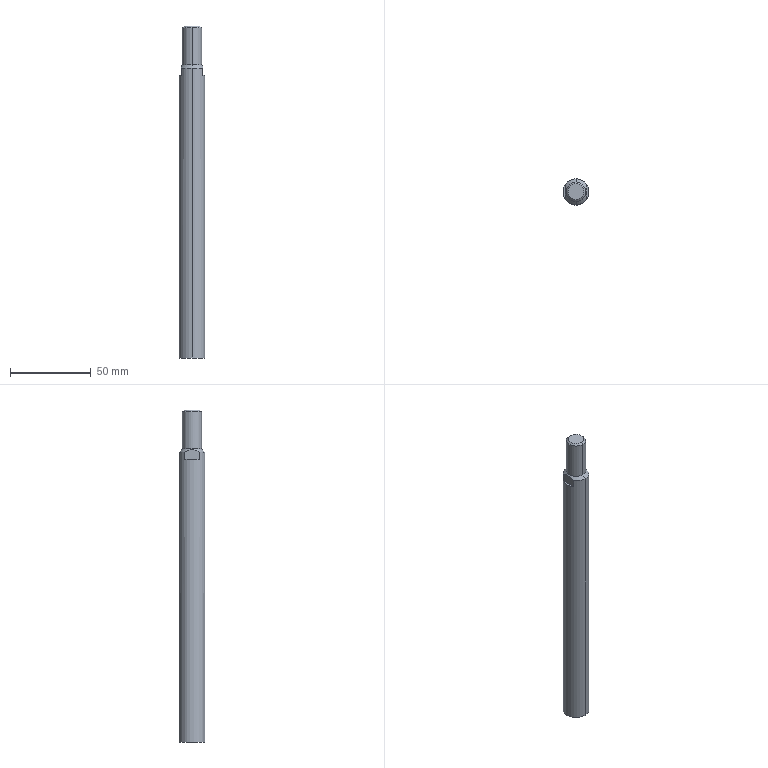Part | STEP file | 1 solid | 14 faces | box 16 x 16 x 205 mm | volume 38897 mm3 | plane 6 | cylinder 4 | cone 4 | commonest cylinder face diameters 12 x2 16 x2
STEP:
#1=CARTESIAN_POINT('',(0.,-8.,-151.));
#2=VERTEX_POINT('',#1);
#3=CARTESIAN_POINT('',(0.,8.,-151.));
#4=VERTEX_POINT('',#3);
#5=CARTESIAN_POINT('',(0.,0.,-151.));
#6=DIRECTION('',(0.,0.,1.));
#7=DIRECTION('',(0.,-1.,0.));
#8=AXIS2_PLACEMENT_3D('',#5,#6,#7);
#9=CIRCLE('',#8,8.);
#10=EDGE_CURVE('',#2,#4,#9,.T.);
#11=ORIENTED_EDGE('',*,*,#10,.T.);
#12=CARTESIAN_POINT('',(0.,8.,28.));
#13=VERTEX_POINT('',#12);
#14=CARTESIAN_POINT('',(0.,8.,-151.));
#15=DIRECTION('',(0.,0.,1.));
#16=VECTOR('',#15,1000.);
#17=LINE('',#14,#16);
#18=EDGE_CURVE('',#4,#13,#17,.T.);
#19=ORIENTED_EDGE('',*,*,#18,.T.);
#20=CARTESIAN_POINT('',(6.5,4.664,28.));
#21=VERTEX_POINT('',#20);
#22=CARTESIAN_POINT('',(0.,0.,28.));
#23=DIRECTION('',(0.,0.,1.));
#24=DIRECTION('',(0.,-1.,0.));
#25=AXIS2_PLACEMENT_3D('',#22,#23,#24);
#26=CIRCLE('',#25,8.);
#27=EDGE_CURVE('',#21,#13,#26,.T.);
#28=ORIENTED_EDGE('',*,*,#27,.F.);
#29=CARTESIAN_POINT('',(6.5,4.664,23.5));
#30=VERTEX_POINT('',#29);
#31=CARTESIAN_POINT('',(6.5,4.664,-151.));
#32=DIRECTION('',(0.,0.,-1.));
#33=VECTOR('',#32,1000.);
#34=LINE('',#31,#33);
#35=EDGE_CURVE('',#21,#30,#34,.T.);
#36=ORIENTED_EDGE('',*,*,#35,.T.);
#37=CARTESIAN_POINT('',(6.5,-4.664,23.5));
#38=VERTEX_POINT('',#37);
#39=CARTESIAN_POINT('',(0.,0.,23.5));
#40=DIRECTION('',(0.,0.,1.));
#41=DIRECTION('',(1.,0.,0.));
#42=AXIS2_PLACEMENT_3D('',#39,#40,#41);
#43=CIRCLE('',#42,8.);
#44=EDGE_CURVE('',#38,#30,#43,.T.);
#45=ORIENTED_EDGE('',*,*,#44,.F.);
#46=CARTESIAN_POINT('',(6.5,-4.664,28.));
#47=VERTEX_POINT('',#46);
#48=CARTESIAN_POINT('',(6.5,-4.664,-151.));
#49=DIRECTION('',(0.,0.,1.));
#50=VECTOR('',#49,1000.);
#51=LINE('',#48,#50);
#52=EDGE_CURVE('',#38,#47,#51,.T.);
#53=ORIENTED_EDGE('',*,*,#52,.T.);
#54=CARTESIAN_POINT('',(0.,-8.,28.));
#55=VERTEX_POINT('',#54);
#56=CARTESIAN_POINT('',(0.,0.,28.));
#57=DIRECTION('',(0.,0.,1.));
#58=DIRECTION('',(0.,-1.,0.));
#59=AXIS2_PLACEMENT_3D('',#56,#57,#58);
#60=CIRCLE('',#59,8.);
#61=EDGE_CURVE('',#55,#47,#60,.T.);
#62=ORIENTED_EDGE('',*,*,#61,.F.);
#63=CARTESIAN_POINT('',(0.,-8.,-151.));
#64=DIRECTION('',(0.,0.,1.));
#65=VECTOR('',#64,1000.);
#66=LINE('',#63,#65);
#67=EDGE_CURVE('',#2,#55,#66,.T.);
#68=ORIENTED_EDGE('',*,*,#67,.F.);
#69=EDGE_LOOP('',(#11,#19,#28,#36,#45,#53,#62,#68));
#70=FACE_OUTER_BOUND('',#69,.T.);
#71=CARTESIAN_POINT('',(0.,0.,-151.));
#72=DIRECTION('',(0.,0.,1.));
#73=DIRECTION('',(0.,-1.,0.));
#74=AXIS2_PLACEMENT_3D('',#71,#72,#73);
#75=CYLINDRICAL_SURFACE('',#74,8.);
#76=ADVANCED_FACE('',(#70),#75,.T.);
#77=CARTESIAN_POINT('',(0.,-6.,30.));
#78=VERTEX_POINT('',#77);
#79=CARTESIAN_POINT('',(0.,6.,30.));
#80=VERTEX_POINT('',#79);
#81=CARTESIAN_POINT('',(0.,0.,30.));
#82=DIRECTION('',(0.,0.,1.));
#83=DIRECTION('',(0.,-1.,0.));
#84=AXIS2_PLACEMENT_3D('',#81,#82,#83);
#85=CIRCLE('',#84,6.);
#86=EDGE_CURVE('',#78,#80,#85,.T.);
#87=ORIENTED_EDGE('',*,*,#86,.F.);
#88=CARTESIAN_POINT('',(0.,-8.,28.));
#89=DIRECTION('',(0.,-0.7071,-0.7071));
#90=VECTOR('',#89,1000.);
#91=LINE('',#88,#90);
#92=EDGE_CURVE('',#78,#55,#91,.T.);
#93=ORIENTED_EDGE('',*,*,#92,.T.);
#94=ORIENTED_EDGE('',*,*,#61,.T.);
#95=CARTESIAN_POINT('',(6.5,-4.664,28.));
#96=CARTESIAN_POINT('',(6.5,-3.949,28.416));
#97=CARTESIAN_POINT('',(6.5,-3.213,28.786));
#98=CARTESIAN_POINT('',(6.5,-2.041,29.197));
#99=CARTESIAN_POINT('',(6.5,-1.637,29.309));
#100=CARTESIAN_POINT('',(6.5,-0.8259,29.46));
#101=CARTESIAN_POINT('',(6.5,-0.4161,29.5));
#102=CARTESIAN_POINT('',(6.5,0.2054,29.5));
#103=CARTESIAN_POINT('',(6.5,0.4149,29.49));
#104=CARTESIAN_POINT('',(6.5,0.829,29.451));
#105=CARTESIAN_POINT('',(6.5,1.034,29.421));
#106=CARTESIAN_POINT('',(6.5,1.643,29.308));
#107=CARTESIAN_POINT('',(6.5,2.041,29.197));
#108=CARTESIAN_POINT('',(6.5,2.824,28.922));
#109=CARTESIAN_POINT('',(6.5,3.207,28.759));
#110=CARTESIAN_POINT('',(6.5,3.949,28.401));
#111=CARTESIAN_POINT('',(6.5,4.31,28.206));
#112=CARTESIAN_POINT('',(6.5,4.664,28.));
#113=B_SPLINE_CURVE_WITH_KNOTS('',3,(#95,#96,#97,#98,#99,#100,#101,#102,#103,#104,#105,#106,#107,#108,#109,#110,#111,#112),.UNSPECIFIED.,.F.,.F.,(4,2,2,2,2,2,2,2,4),(0.01031,0.01278,0.01401,0.01525,0.01587,0.01648,0.01772,0.01896,0.02019),.UNSPECIFIED.);
#114=EDGE_CURVE('',#47,#21,#113,.T.);
#115=ORIENTED_EDGE('',*,*,#114,.T.);
#116=ORIENTED_EDGE('',*,*,#27,.T.);
#117=CARTESIAN_POINT('',(0.,8.,28.));
#118=DIRECTION('',(0.,0.7071,-0.7071));
#119=VECTOR('',#118,1000.);
#120=LINE('',#117,#119);
#121=EDGE_CURVE('',#80,#13,#120,.T.);
#122=ORIENTED_EDGE('',*,*,#121,.F.);
#123=EDGE_LOOP('',(#87,#93,#94,#115,#116,#122));
#124=FACE_OUTER_BOUND('',#123,.T.);
#125=CARTESIAN_POINT('',(0.,0.,28.));
#126=DIRECTION('',(0.,0.,-1.));
#127=DIRECTION('',(0.,1.,0.));
#128=AXIS2_PLACEMENT_3D('',#125,#126,#127);
#129=CONICAL_SURFACE('',#128,8.,0.7854);
#130=ADVANCED_FACE('',(#124),#129,.T.);
#131=ORIENTED_EDGE('',*,*,#86,.T.);
#132=CARTESIAN_POINT('',(0.,6.,52.927));
#133=VERTEX_POINT('',#132);
#134=CARTESIAN_POINT('',(0.,6.,-151.));
#135=DIRECTION('',(0.,0.,1.));
#136=VECTOR('',#135,1000.);
#137=LINE('',#134,#136);
#138=EDGE_CURVE('',#80,#133,#137,.T.);
#139=ORIENTED_EDGE('',*,*,#138,.T.);
#140=CARTESIAN_POINT('',(0.,-6.,52.927));
#141=VERTEX_POINT('',#140);
#142=CARTESIAN_POINT('',(0.,0.,52.927));
#143=DIRECTION('',(0.,0.,1.));
#144=DIRECTION('',(0.,-1.,0.));
#145=AXIS2_PLACEMENT_3D('',#142,#143,#144);
#146=CIRCLE('',#145,6.);
#147=EDGE_CURVE('',#141,#133,#146,.T.);
#148=ORIENTED_EDGE('',*,*,#147,.F.);
#149=CARTESIAN_POINT('',(0.,-6.,-151.));
#150=DIRECTION('',(0.,0.,1.));
#151=VECTOR('',#150,1000.);
#152=LINE('',#149,#151);
#153=EDGE_CURVE('',#78,#141,#152,.T.);
#154=ORIENTED_EDGE('',*,*,#153,.F.);
#155=EDGE_LOOP('',(#131,#139,#148,#154));
#156=FACE_OUTER_BOUND('',#155,.T.);
#157=CARTESIAN_POINT('',(0.,0.,-151.));
#158=DIRECTION('',(0.,0.,1.));
#159=DIRECTION('',(0.,-1.,0.));
#160=AXIS2_PLACEMENT_3D('',#157,#158,#159);
#161=CYLINDRICAL_SURFACE('',#160,6.);
#162=ADVANCED_FACE('',(#156),#161,.T.);
#163=CARTESIAN_POINT('',(0.,-4.926,54.));
#164=VERTEX_POINT('',#163);
#165=CARTESIAN_POINT('',(0.,4.926,54.));
#166=VERTEX_POINT('',#165);
#167=CARTESIAN_POINT('',(0.,0.,54.));
#168=DIRECTION('',(0.,0.,1.));
#169=DIRECTION('',(0.,-1.,0.));
#170=AXIS2_PLACEMENT_3D('',#167,#168,#169);
#171=CIRCLE('',#170,4.926);
#172=EDGE_CURVE('',#164,#166,#171,.T.);
#173=ORIENTED_EDGE('',*,*,#172,.F.);
#174=CARTESIAN_POINT('',(0.,-6.,52.927));
#175=DIRECTION('',(0.,-0.7071,-0.7071));
#176=VECTOR('',#175,1000.);
#177=LINE('',#174,#176);
#178=EDGE_CURVE('',#164,#141,#177,.T.);
#179=ORIENTED_EDGE('',*,*,#178,.T.);
#180=ORIENTED_EDGE('',*,*,#147,.T.);
#181=CARTESIAN_POINT('',(0.,6.,52.927));
#182=DIRECTION('',(0.,0.7071,-0.7071));
#183=VECTOR('',#182,1000.);
#184=LINE('',#181,#183);
#185=EDGE_CURVE('',#166,#133,#184,.T.);
#186=ORIENTED_EDGE('',*,*,#185,.F.);
#187=EDGE_LOOP('',(#173,#179,#180,#186));
#188=FACE_OUTER_BOUND('',#187,.T.);
#189=CARTESIAN_POINT('',(0.,0.,52.927));
#190=DIRECTION('',(0.,0.,-1.));
#191=DIRECTION('',(0.,1.,0.));
#192=AXIS2_PLACEMENT_3D('',#189,#190,#191);
#193=CONICAL_SURFACE('',#192,6.,0.7854);
#194=ADVANCED_FACE('',(#188),#193,.T.);
#195=CARTESIAN_POINT('',(0.,0.,54.));
#196=DIRECTION('',(0.,0.,1.));
#197=DIRECTION('',(0.,-1.,0.));
#198=AXIS2_PLACEMENT_3D('',#195,#196,#197);
#199=CIRCLE('',#198,4.926);
#200=EDGE_CURVE('',#166,#164,#199,.T.);
#201=ORIENTED_EDGE('',*,*,#200,.T.);
#202=ORIENTED_EDGE('',*,*,#172,.T.);
#203=EDGE_LOOP('',(#201,#202));
#204=FACE_OUTER_BOUND('',#203,.T.);
#205=CARTESIAN_POINT('',(0.,0.,54.));
#206=DIRECTION('',(0.,0.,-1.));
#207=DIRECTION('',(0.,1.,0.));
#208=AXIS2_PLACEMENT_3D('',#205,#206,#207);
#209=PLANE('',#208);
#210=ADVANCED_FACE('',(#204),#209,.F.);
#211=ORIENTED_EDGE('',*,*,#178,.F.);
#212=ORIENTED_EDGE('',*,*,#200,.F.);
#213=ORIENTED_EDGE('',*,*,#185,.T.);
#214=CARTESIAN_POINT('',(0.,0.,52.927));
#215=DIRECTION('',(0.,0.,1.));
#216=DIRECTION('',(0.,-1.,0.));
#217=AXIS2_PLACEMENT_3D('',#214,#215,#216);
#218=CIRCLE('',#217,6.);
#219=EDGE_CURVE('',#133,#141,#218,.T.);
#220=ORIENTED_EDGE('',*,*,#219,.T.);
#221=EDGE_LOOP('',(#211,#212,#213,#220));
#222=FACE_OUTER_BOUND('',#221,.T.);
#223=CARTESIAN_POINT('',(0.,0.,52.927));
#224=DIRECTION('',(0.,0.,-1.));
#225=DIRECTION('',(0.,1.,0.));
#226=AXIS2_PLACEMENT_3D('',#223,#224,#225);
#227=CONICAL_SURFACE('',#226,6.,0.7854);
#228=ADVANCED_FACE('',(#222),#227,.T.);
#229=ORIENTED_EDGE('',*,*,#138,.F.);
#230=CARTESIAN_POINT('',(0.,0.,30.));
#231=DIRECTION('',(0.,0.,1.));
#232=DIRECTION('',(0.,-1.,0.));
#233=AXIS2_PLACEMENT_3D('',#230,#231,#232);
#234=CIRCLE('',#233,6.);
#235=EDGE_CURVE('',#80,#78,#234,.T.);
#236=ORIENTED_EDGE('',*,*,#235,.T.);
#237=ORIENTED_EDGE('',*,*,#153,.T.);
#238=ORIENTED_EDGE('',*,*,#219,.F.);
#239=EDGE_LOOP('',(#229,#236,#237,#238));
#240=FACE_OUTER_BOUND('',#239,.T.);
#241=CARTESIAN_POINT('',(0.,0.,-151.));
#242=DIRECTION('',(0.,0.,1.));
#243=DIRECTION('',(0.,-1.,0.));
#244=AXIS2_PLACEMENT_3D('',#241,#242,#243);
#245=CYLINDRICAL_SURFACE('',#244,6.);
#246=ADVANCED_FACE('',(#240),#245,.T.);
#247=ORIENTED_EDGE('',*,*,#92,.F.);
#248=ORIENTED_EDGE('',*,*,#235,.F.);
#249=ORIENTED_EDGE('',*,*,#121,.T.);
#250=CARTESIAN_POINT('',(-6.5,4.664,28.));
#251=VERTEX_POINT('',#250);
#252=CARTESIAN_POINT('',(0.,0.,28.));
#253=DIRECTION('',(0.,0.,1.));
#254=DIRECTION('',(0.,-1.,0.));
#255=AXIS2_PLACEMENT_3D('',#252,#253,#254);
#256=CIRCLE('',#255,8.);
#257=EDGE_CURVE('',#13,#251,#256,.T.);
#258=ORIENTED_EDGE('',*,*,#257,.T.);
#259=CARTESIAN_POINT('',(-6.5,-4.664,28.));
#260=VERTEX_POINT('',#259);
#261=CARTESIAN_POINT('',(-6.5,4.664,28.));
#262=CARTESIAN_POINT('',(-6.5,4.31,28.206));
#263=CARTESIAN_POINT('',(-6.5,3.949,28.401));
#264=CARTESIAN_POINT('',(-6.5,3.207,28.759));
#265=CARTESIAN_POINT('',(-6.5,2.824,28.922));
#266=CARTESIAN_POINT('',(-6.5,2.041,29.197));
#267=CARTESIAN_POINT('',(-6.5,1.643,29.308));
#268=CARTESIAN_POINT('',(-6.5,1.034,29.421));
#269=CARTESIAN_POINT('',(-6.5,0.829,29.451));
#270=CARTESIAN_POINT('',(-6.5,0.4149,29.49));
#271=CARTESIAN_POINT('',(-6.5,0.2054,29.5));
#272=CARTESIAN_POINT('',(-6.5,-0.4161,29.5));
#273=CARTESIAN_POINT('',(-6.5,-0.8259,29.46));
#274=CARTESIAN_POINT('',(-6.5,-1.637,29.309));
#275=CARTESIAN_POINT('',(-6.5,-2.041,29.197));
#276=CARTESIAN_POINT('',(-6.5,-3.213,28.786));
#277=CARTESIAN_POINT('',(-6.5,-3.949,28.416));
#278=CARTESIAN_POINT('',(-6.5,-4.664,28.));
#279=B_SPLINE_CURVE_WITH_KNOTS('',3,(#261,#262,#263,#264,#265,#266,#267,#268,#269,#270,#271,#272,#273,#274,#275,#276,#277,#278),.UNSPECIFIED.,.F.,.F.,(4,2,2,2,2,2,2,2,4),(0.003921,0.005149,0.006378,0.007607,0.008221,0.008835,0.01006,0.01129,0.01375),.UNSPECIFIED.);
#280=EDGE_CURVE('',#251,#260,#279,.T.);
#281=ORIENTED_EDGE('',*,*,#280,.T.);
#282=CARTESIAN_POINT('',(0.,0.,28.));
#283=DIRECTION('',(0.,0.,1.));
#284=DIRECTION('',(0.,-1.,0.));
#285=AXIS2_PLACEMENT_3D('',#282,#283,#284);
#286=CIRCLE('',#285,8.);
#287=EDGE_CURVE('',#260,#55,#286,.T.);
#288=ORIENTED_EDGE('',*,*,#287,.T.);
#289=EDGE_LOOP('',(#247,#248,#249,#258,#281,#288));
#290=FACE_OUTER_BOUND('',#289,.T.);
#291=CARTESIAN_POINT('',(0.,0.,28.));
#292=DIRECTION('',(0.,0.,-1.));
#293=DIRECTION('',(0.,1.,0.));
#294=AXIS2_PLACEMENT_3D('',#291,#292,#293);
#295=CONICAL_SURFACE('',#294,8.,0.7854);
#296=ADVANCED_FACE('',(#290),#295,.T.);
#297=ORIENTED_EDGE('',*,*,#18,.F.);
#298=CARTESIAN_POINT('',(0.,0.,-151.));
#299=DIRECTION('',(0.,0.,1.));
#300=DIRECTION('',(0.,-1.,0.));
#301=AXIS2_PLACEMENT_3D('',#298,#299,#300);
#302=CIRCLE('',#301,8.);
#303=EDGE_CURVE('',#4,#2,#302,.T.);
#304=ORIENTED_EDGE('',*,*,#303,.T.);
#305=ORIENTED_EDGE('',*,*,#67,.T.);
#306=ORIENTED_EDGE('',*,*,#287,.F.);
#307=CARTESIAN_POINT('',(-6.5,-4.664,23.5));
#308=VERTEX_POINT('',#307);
#309=CARTESIAN_POINT('',(-6.5,-4.664,-151.));
#310=DIRECTION('',(0.,0.,-1.));
#311=VECTOR('',#310,1000.);
#312=LINE('',#309,#311);
#313=EDGE_CURVE('',#260,#308,#312,.T.);
#314=ORIENTED_EDGE('',*,*,#313,.T.);
#315=CARTESIAN_POINT('',(-6.5,4.664,23.5));
#316=VERTEX_POINT('',#315);
#317=CARTESIAN_POINT('',(0.,0.,23.5));
#318=DIRECTION('',(0.,0.,1.));
#319=DIRECTION('',(1.,0.,0.));
#320=AXIS2_PLACEMENT_3D('',#317,#318,#319);
#321=CIRCLE('',#320,8.);
#322=EDGE_CURVE('',#316,#308,#321,.T.);
#323=ORIENTED_EDGE('',*,*,#322,.F.);
#324=CARTESIAN_POINT('',(-6.5,4.664,-151.));
#325=DIRECTION('',(0.,0.,1.));
#326=VECTOR('',#325,1000.);
#327=LINE('',#324,#326);
#328=EDGE_CURVE('',#316,#251,#327,.T.);
#329=ORIENTED_EDGE('',*,*,#328,.T.);
#330=ORIENTED_EDGE('',*,*,#257,.F.);
#331=EDGE_LOOP('',(#297,#304,#305,#306,#314,#323,#329,#330));
#332=FACE_OUTER_BOUND('',#331,.T.);
#333=CARTESIAN_POINT('',(0.,0.,-151.));
#334=DIRECTION('',(0.,0.,1.));
#335=DIRECTION('',(0.,-1.,0.));
#336=AXIS2_PLACEMENT_3D('',#333,#334,#335);
#337=CYLINDRICAL_SURFACE('',#336,8.);
#338=ADVANCED_FACE('',(#332),#337,.T.);
#339=ORIENTED_EDGE('',*,*,#10,.F.);
#340=ORIENTED_EDGE('',*,*,#303,.F.);
#341=EDGE_LOOP('',(#339,#340));
#342=FACE_OUTER_BOUND('',#341,.T.);
#343=CARTESIAN_POINT('',(0.,8.,-151.));
#344=DIRECTION('',(0.,0.,1.));
#345=DIRECTION('',(0.,-1.,0.));
#346=AXIS2_PLACEMENT_3D('',#343,#344,#345);
#347=PLANE('',#346);
#348=ADVANCED_FACE('',(#342),#347,.F.);
#349=ORIENTED_EDGE('',*,*,#44,.T.);
#350=CARTESIAN_POINT('',(6.5,17.5,23.5));
#351=DIRECTION('',(0.,-1.,0.));
#352=VECTOR('',#351,1000.);
#353=LINE('',#350,#352);
#354=EDGE_CURVE('',#30,#38,#353,.T.);
#355=ORIENTED_EDGE('',*,*,#354,.T.);
#356=EDGE_LOOP('',(#349,#355));
#357=FACE_OUTER_BOUND('',#356,.T.);
#358=CARTESIAN_POINT('',(-16.5,-17.5,23.5));
#359=DIRECTION('',(0.,0.,1.));
#360=DIRECTION('',(1.,0.,0.));
#361=AXIS2_PLACEMENT_3D('',#358,#359,#360);
#362=PLANE('',#361);
#363=ADVANCED_FACE('',(#357),#362,.T.);
#364=ORIENTED_EDGE('',*,*,#354,.F.);
#365=ORIENTED_EDGE('',*,*,#35,.F.);
#366=ORIENTED_EDGE('',*,*,#114,.F.);
#367=ORIENTED_EDGE('',*,*,#52,.F.);
#368=EDGE_LOOP('',(#364,#365,#366,#367));
#369=FACE_OUTER_BOUND('',#368,.T.);
#370=CARTESIAN_POINT('',(6.5,17.5,23.5));
#371=DIRECTION('',(-1.,0.,0.));
#372=DIRECTION('',(0.,0.,1.));
#373=AXIS2_PLACEMENT_3D('',#370,#371,#372);
#374=PLANE('',#373);
#375=ADVANCED_FACE('',(#369),#374,.F.);
#376=CARTESIAN_POINT('',(-6.5,-17.5,23.5));
#377=DIRECTION('',(0.,1.,0.));
#378=VECTOR('',#377,1000.);
#379=LINE('',#376,#378);
#380=EDGE_CURVE('',#308,#316,#379,.T.);
#381=ORIENTED_EDGE('',*,*,#380,.F.);
#382=ORIENTED_EDGE('',*,*,#313,.F.);
#383=ORIENTED_EDGE('',*,*,#280,.F.);
#384=ORIENTED_EDGE('',*,*,#328,.F.);
#385=EDGE_LOOP('',(#381,#382,#383,#384));
#386=FACE_OUTER_BOUND('',#385,.T.);
#387=CARTESIAN_POINT('',(-6.5,-17.5,23.5));
#388=DIRECTION('',(1.,0.,0.));
#389=DIRECTION('',(0.,0.,-1.));
#390=AXIS2_PLACEMENT_3D('',#387,#388,#389);
#391=PLANE('',#390);
#392=ADVANCED_FACE('',(#386),#391,.F.);
#393=ORIENTED_EDGE('',*,*,#322,.T.);
#394=ORIENTED_EDGE('',*,*,#380,.T.);
#395=EDGE_LOOP('',(#393,#394));
#396=FACE_OUTER_BOUND('',#395,.T.);
#397=CARTESIAN_POINT('',(-16.5,-17.5,23.5));
#398=DIRECTION('',(0.,0.,1.));
#399=DIRECTION('',(1.,0.,0.));
#400=AXIS2_PLACEMENT_3D('',#397,#398,#399);
#401=PLANE('',#400);
#402=ADVANCED_FACE('',(#396),#401,.T.);
#403=CLOSED_SHELL('',(#76,#130,#162,#194,#210,#228,#246,#296,#338,#348,#363,#375,#392,#402));
#404=MANIFOLD_SOLID_BREP('',#403);
#405=CARTESIAN_POINT('',(0.,0.,0.));
#406=DIRECTION('',(0.,0.,1.));
#407=DIRECTION('',(1.,0.,0.));
#408=AXIS2_PLACEMENT_3D('',#405,#406,#407);
#409=(LENGTH_UNIT()NAMED_UNIT(*)SI_UNIT(.MILLI.,.METRE.));
#410=UNCERTAINTY_MEASURE_WITH_UNIT(LENGTH_MEASURE(0.00001),#409,'','');
#411=(NAMED_UNIT(*)PLANE_ANGLE_UNIT()SI_UNIT($,.RADIAN.));
#412=(NAMED_UNIT(*)SI_UNIT($,.STERADIAN.)SOLID_ANGLE_UNIT());
#413=(GEOMETRIC_REPRESENTATION_CONTEXT(3)GLOBAL_UNCERTAINTY_ASSIGNED_CONTEXT((#410))GLOBAL_UNIT_ASSIGNED_CONTEXT((#409,#411,#412))REPRESENTATION_CONTEXT('',''));
#414=ADVANCED_BREP_SHAPE_REPRESENTATION('',(#404,#408),#413);